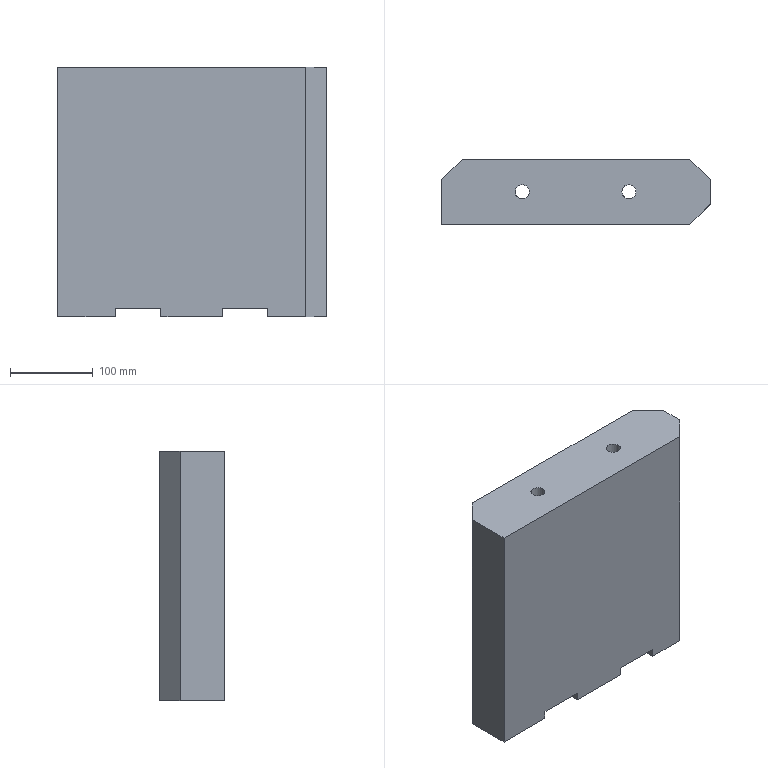Part | NX | features solid 2 | 1 solid | 23 faces | box 325 x 79 x 302 mm | volume 7112988 mm3 | plane 19 | cylinder 4 | commonest cylinder face diameters 17 x2 25 x2
STEP:
#1=CARTESIAN_POINT('',(-50.,-343.,178.));
#2=VERTEX_POINT('',#1);
#3=CARTESIAN_POINT('',(24.,-343.,178.));
#4=VERTEX_POINT('',#3);
#5=CARTESIAN_POINT('',(-177.942,-343.,178.));
#6=DIRECTION('',(1.,0.,0.));
#7=VECTOR('',#6,1000.);
#8=LINE('',#5,#7);
#9=EDGE_CURVE('',#2,#4,#8,.T.);
#10=ORIENTED_EDGE('',*,*,#9,.T.);
#11=CARTESIAN_POINT('',(24.,-422.,178.));
#12=VERTEX_POINT('',#11);
#13=CARTESIAN_POINT('',(24.,-420.217,178.));
#14=DIRECTION('',(0.,-1.,0.));
#15=VECTOR('',#14,1000.);
#16=LINE('',#13,#15);
#17=EDGE_CURVE('',#4,#12,#16,.T.);
#18=ORIENTED_EDGE('',*,*,#17,.T.);
#19=CARTESIAN_POINT('',(-50.,-422.,178.));
#20=VERTEX_POINT('',#19);
#21=CARTESIAN_POINT('',(-117.942,-422.,178.));
#22=DIRECTION('',(-1.,0.,0.));
#23=VECTOR('',#22,1000.);
#24=LINE('',#21,#23);
#25=EDGE_CURVE('',#12,#20,#24,.T.);
#26=ORIENTED_EDGE('',*,*,#25,.T.);
#27=CARTESIAN_POINT('',(-50.,-420.217,178.));
#28=DIRECTION('',(0.,-1.,0.));
#29=VECTOR('',#28,1000.);
#30=LINE('',#27,#29);
#31=EDGE_CURVE('',#2,#20,#30,.T.);
#32=ORIENTED_EDGE('',*,*,#31,.F.);
#33=EDGE_LOOP('',(#10,#18,#26,#32));
#34=FACE_BOUND('',#33,.T.);
#35=CARTESIAN_POINT('',(-177.942,-420.217,178.));
#36=DIRECTION('',(0.,0.,-1.));
#37=DIRECTION('',(0.,1.,0.));
#38=AXIS2_PLACEMENT_3D('',#35,#36,#37);
#39=PLANE('',#38);
#40=ADVANCED_FACE('',(#34),#39,.T.);
#41=CARTESIAN_POINT('',(-150.,-343.,178.));
#42=VERTEX_POINT('',#41);
#43=CARTESIAN_POINT('',(-105.,-343.,178.));
#44=VERTEX_POINT('',#43);
#45=CARTESIAN_POINT('',(-177.942,-343.,178.));
#46=DIRECTION('',(1.,0.,0.));
#47=VECTOR('',#46,1000.);
#48=LINE('',#45,#47);
#49=EDGE_CURVE('',#42,#44,#48,.T.);
#50=ORIENTED_EDGE('',*,*,#49,.T.);
#51=CARTESIAN_POINT('',(-105.,-422.,178.));
#52=VERTEX_POINT('',#51);
#53=CARTESIAN_POINT('',(-105.,-420.217,178.));
#54=DIRECTION('',(0.,-1.,0.));
#55=VECTOR('',#54,1000.);
#56=LINE('',#53,#55);
#57=EDGE_CURVE('',#44,#52,#56,.T.);
#58=ORIENTED_EDGE('',*,*,#57,.T.);
#59=CARTESIAN_POINT('',(-175.,-422.,178.));
#60=VERTEX_POINT('',#59);
#61=CARTESIAN_POINT('',(-117.942,-422.,178.));
#62=DIRECTION('',(-1.,0.,0.));
#63=VECTOR('',#62,1000.);
#64=LINE('',#61,#63);
#65=EDGE_CURVE('',#52,#60,#64,.T.);
#66=ORIENTED_EDGE('',*,*,#65,.T.);
#67=CARTESIAN_POINT('',(-175.,-368.,178.));
#68=VERTEX_POINT('',#67);
#69=CARTESIAN_POINT('',(-175.,-420.217,178.));
#70=DIRECTION('',(0.,1.,0.));
#71=VECTOR('',#70,1000.);
#72=LINE('',#69,#71);
#73=EDGE_CURVE('',#60,#68,#72,.T.);
#74=ORIENTED_EDGE('',*,*,#73,.T.);
#75=CARTESIAN_POINT('',(-202.579,-395.579,178.));
#76=DIRECTION('',(-0.7071,-0.7071,0.));
#77=VECTOR('',#76,1000.);
#78=LINE('',#75,#77);
#79=EDGE_CURVE('',#68,#42,#78,.F.);
#80=ORIENTED_EDGE('',*,*,#79,.T.);
#81=EDGE_LOOP('',(#50,#58,#66,#74,#80));
#82=FACE_BOUND('',#81,.T.);
#83=CARTESIAN_POINT('',(-177.942,-420.217,178.));
#84=DIRECTION('',(0.,0.,-1.));
#85=DIRECTION('',(0.,1.,0.));
#86=AXIS2_PLACEMENT_3D('',#83,#84,#85);
#87=PLANE('',#86);
#88=ADVANCED_FACE('',(#82),#87,.T.);
#89=CARTESIAN_POINT('',(24.,-422.,188.));
#90=VERTEX_POINT('',#89);
#91=CARTESIAN_POINT('',(79.,-422.,188.));
#92=VERTEX_POINT('',#91);
#93=CARTESIAN_POINT('',(24.489,-422.,188.));
#94=DIRECTION('',(-1.,0.,0.));
#95=VECTOR('',#94,1000.);
#96=LINE('',#93,#95);
#97=EDGE_CURVE('',#90,#92,#96,.F.);
#98=ORIENTED_EDGE('',*,*,#97,.T.);
#99=CARTESIAN_POINT('',(79.,-422.,178.));
#100=VERTEX_POINT('',#99);
#101=CARTESIAN_POINT('',(79.,-422.,192.6));
#102=DIRECTION('',(0.,0.,-1.));
#103=VECTOR('',#102,1000.);
#104=LINE('',#101,#103);
#105=EDGE_CURVE('',#92,#100,#104,.T.);
#106=ORIENTED_EDGE('',*,*,#105,.T.);
#107=CARTESIAN_POINT('',(125.,-422.,178.));
#108=VERTEX_POINT('',#107);
#109=CARTESIAN_POINT('',(-117.942,-422.,178.));
#110=DIRECTION('',(-1.,0.,0.));
#111=VECTOR('',#110,1000.);
#112=LINE('',#109,#111);
#113=EDGE_CURVE('',#108,#100,#112,.T.);
#114=ORIENTED_EDGE('',*,*,#113,.F.);
#115=CARTESIAN_POINT('',(125.,-422.,480.));
#116=VERTEX_POINT('',#115);
#117=CARTESIAN_POINT('',(125.,-422.,480.));
#118=DIRECTION('',(0.,0.,1.));
#119=VECTOR('',#118,1000.);
#120=LINE('',#117,#119);
#121=EDGE_CURVE('',#108,#116,#120,.T.);
#122=ORIENTED_EDGE('',*,*,#121,.T.);
#123=CARTESIAN_POINT('',(-175.,-422.,480.));
#124=VERTEX_POINT('',#123);
#125=CARTESIAN_POINT('',(-117.942,-422.,480.));
#126=DIRECTION('',(1.,0.,0.));
#127=VECTOR('',#126,1000.);
#128=LINE('',#125,#127);
#129=EDGE_CURVE('',#116,#124,#128,.F.);
#130=ORIENTED_EDGE('',*,*,#129,.T.);
#131=CARTESIAN_POINT('',(-175.,-422.,192.6));
#132=DIRECTION('',(0.,0.,1.));
#133=VECTOR('',#132,1000.);
#134=LINE('',#131,#133);
#135=EDGE_CURVE('',#60,#124,#134,.T.);
#136=ORIENTED_EDGE('',*,*,#135,.F.);
#137=ORIENTED_EDGE('',*,*,#65,.F.);
#138=CARTESIAN_POINT('',(-105.,-422.,188.));
#139=VERTEX_POINT('',#138);
#140=CARTESIAN_POINT('',(-105.,-422.,192.6));
#141=DIRECTION('',(0.,0.,-1.));
#142=VECTOR('',#141,1000.);
#143=LINE('',#140,#142);
#144=EDGE_CURVE('',#139,#52,#143,.T.);
#145=ORIENTED_EDGE('',*,*,#144,.F.);
#146=CARTESIAN_POINT('',(-50.,-422.,188.));
#147=VERTEX_POINT('',#146);
#148=CARTESIAN_POINT('',(-105.511,-422.,188.));
#149=DIRECTION('',(-1.,0.,0.));
#150=VECTOR('',#149,1000.);
#151=LINE('',#148,#150);
#152=EDGE_CURVE('',#139,#147,#151,.F.);
#153=ORIENTED_EDGE('',*,*,#152,.T.);
#154=CARTESIAN_POINT('',(-50.,-422.,192.6));
#155=DIRECTION('',(0.,0.,-1.));
#156=VECTOR('',#155,1000.);
#157=LINE('',#154,#156);
#158=EDGE_CURVE('',#147,#20,#157,.T.);
#159=ORIENTED_EDGE('',*,*,#158,.T.);
#160=ORIENTED_EDGE('',*,*,#25,.F.);
#161=CARTESIAN_POINT('',(24.,-422.,192.6));
#162=DIRECTION('',(0.,0.,-1.));
#163=VECTOR('',#162,1000.);
#164=LINE('',#161,#163);
#165=EDGE_CURVE('',#90,#12,#164,.T.);
#166=ORIENTED_EDGE('',*,*,#165,.F.);
#167=EDGE_LOOP('',(#98,#106,#114,#122,#130,#136,#137,#145,#153,#159,#160,#166));
#168=FACE_BOUND('',#167,.T.);
#169=CARTESIAN_POINT('',(-117.942,-422.,192.6));
#170=DIRECTION('',(0.,1.,0.));
#171=DIRECTION('',(0.,0.,1.));
#172=AXIS2_PLACEMENT_3D('',#169,#170,#171);
#173=PLANE('',#172);
#174=ADVANCED_FACE('',(#168),#173,.F.);
#175=CARTESIAN_POINT('',(-175.,-368.,480.));
#176=VERTEX_POINT('',#175);
#177=CARTESIAN_POINT('',(-175.,-420.217,480.));
#178=DIRECTION('',(0.,-1.,0.));
#179=VECTOR('',#178,1000.);
#180=LINE('',#177,#179);
#181=EDGE_CURVE('',#124,#176,#180,.F.);
#182=ORIENTED_EDGE('',*,*,#181,.T.);
#183=CARTESIAN_POINT('',(-175.,-368.,192.6));
#184=DIRECTION('',(0.,0.,-1.));
#185=VECTOR('',#184,1000.);
#186=LINE('',#183,#185);
#187=EDGE_CURVE('',#176,#68,#186,.T.);
#188=ORIENTED_EDGE('',*,*,#187,.T.);
#189=ORIENTED_EDGE('',*,*,#73,.F.);
#190=ORIENTED_EDGE('',*,*,#135,.T.);
#191=EDGE_LOOP('',(#182,#188,#189,#190));
#192=FACE_BOUND('',#191,.T.);
#193=CARTESIAN_POINT('',(-175.,-420.217,192.6));
#194=DIRECTION('',(1.,0.,0.));
#195=DIRECTION('',(0.,0.,-1.));
#196=AXIS2_PLACEMENT_3D('',#193,#194,#195);
#197=PLANE('',#196);
#198=ADVANCED_FACE('',(#192),#197,.F.);
#199=CARTESIAN_POINT('',(79.,-343.,178.));
#200=VERTEX_POINT('',#199);
#201=CARTESIAN_POINT('',(125.,-343.,178.));
#202=VERTEX_POINT('',#201);
#203=CARTESIAN_POINT('',(-177.942,-343.,178.));
#204=DIRECTION('',(1.,0.,0.));
#205=VECTOR('',#204,1000.);
#206=LINE('',#203,#205);
#207=EDGE_CURVE('',#200,#202,#206,.T.);
#208=ORIENTED_EDGE('',*,*,#207,.F.);
#209=CARTESIAN_POINT('',(79.,-343.,188.));
#210=VERTEX_POINT('',#209);
#211=CARTESIAN_POINT('',(79.,-343.,193.));
#212=DIRECTION('',(0.,0.,-1.));
#213=VECTOR('',#212,1000.);
#214=LINE('',#211,#213);
#215=EDGE_CURVE('',#210,#200,#214,.T.);
#216=ORIENTED_EDGE('',*,*,#215,.F.);
#217=CARTESIAN_POINT('',(24.,-343.,188.));
#218=VERTEX_POINT('',#217);
#219=CARTESIAN_POINT('',(-177.942,-343.,188.));
#220=DIRECTION('',(-1.,0.,0.));
#221=VECTOR('',#220,1000.);
#222=LINE('',#219,#221);
#223=EDGE_CURVE('',#218,#210,#222,.F.);
#224=ORIENTED_EDGE('',*,*,#223,.F.);
#225=CARTESIAN_POINT('',(24.,-343.,193.));
#226=DIRECTION('',(0.,0.,-1.));
#227=VECTOR('',#226,1000.);
#228=LINE('',#225,#227);
#229=EDGE_CURVE('',#218,#4,#228,.T.);
#230=ORIENTED_EDGE('',*,*,#229,.T.);
#231=ORIENTED_EDGE('',*,*,#9,.F.);
#232=CARTESIAN_POINT('',(-50.,-343.,188.));
#233=VERTEX_POINT('',#232);
#234=CARTESIAN_POINT('',(-50.,-343.,193.));
#235=DIRECTION('',(0.,0.,-1.));
#236=VECTOR('',#235,1000.);
#237=LINE('',#234,#236);
#238=EDGE_CURVE('',#233,#2,#237,.T.);
#239=ORIENTED_EDGE('',*,*,#238,.F.);
#240=CARTESIAN_POINT('',(-105.,-343.,188.));
#241=VERTEX_POINT('',#240);
#242=CARTESIAN_POINT('',(-177.942,-343.,188.));
#243=DIRECTION('',(-1.,0.,0.));
#244=VECTOR('',#243,1000.);
#245=LINE('',#242,#244);
#246=EDGE_CURVE('',#241,#233,#245,.F.);
#247=ORIENTED_EDGE('',*,*,#246,.F.);
#248=CARTESIAN_POINT('',(-105.,-343.,193.));
#249=DIRECTION('',(0.,0.,-1.));
#250=VECTOR('',#249,1000.);
#251=LINE('',#248,#250);
#252=EDGE_CURVE('',#241,#44,#251,.T.);
#253=ORIENTED_EDGE('',*,*,#252,.T.);
#254=ORIENTED_EDGE('',*,*,#49,.F.);
#255=CARTESIAN_POINT('',(-150.,-343.,480.));
#256=VERTEX_POINT('',#255);
#257=CARTESIAN_POINT('',(-150.,-343.,192.6));
#258=DIRECTION('',(0.,0.,1.));
#259=VECTOR('',#258,1000.);
#260=LINE('',#257,#259);
#261=EDGE_CURVE('',#42,#256,#260,.T.);
#262=ORIENTED_EDGE('',*,*,#261,.T.);
#263=CARTESIAN_POINT('',(125.,-343.,480.));
#264=VERTEX_POINT('',#263);
#265=CARTESIAN_POINT('',(-177.942,-343.,480.));
#266=DIRECTION('',(-1.,0.,0.));
#267=VECTOR('',#266,1000.);
#268=LINE('',#265,#267);
#269=EDGE_CURVE('',#256,#264,#268,.F.);
#270=ORIENTED_EDGE('',*,*,#269,.T.);
#271=CARTESIAN_POINT('',(125.,-343.,178.));
#272=DIRECTION('',(0.,0.,-1.));
#273=VECTOR('',#272,1000.);
#274=LINE('',#271,#273);
#275=EDGE_CURVE('',#264,#202,#274,.T.);
#276=ORIENTED_EDGE('',*,*,#275,.T.);
#277=EDGE_LOOP('',(#208,#216,#224,#230,#231,#239,#247,#253,#254,#262,#270,#276));
#278=FACE_BOUND('',#277,.T.);
#279=CARTESIAN_POINT('',(-177.942,-343.,192.6));
#280=DIRECTION('',(0.,-1.,0.));
#281=DIRECTION('',(0.,0.,-1.));
#282=AXIS2_PLACEMENT_3D('',#279,#280,#281);
#283=PLANE('',#282);
#284=ADVANCED_FACE('',(#278),#283,.F.);
#285=CARTESIAN_POINT('',(150.,-397.,178.));
#286=VERTEX_POINT('',#285);
#287=CARTESIAN_POINT('',(150.,-368.,178.));
#288=VERTEX_POINT('',#287);
#289=CARTESIAN_POINT('',(150.,-420.217,178.));
#290=DIRECTION('',(0.,1.,0.));
#291=VECTOR('',#290,1000.);
#292=LINE('',#289,#291);
#293=EDGE_CURVE('',#286,#288,#292,.T.);
#294=ORIENTED_EDGE('',*,*,#293,.T.);
#295=CARTESIAN_POINT('',(150.,-368.,480.));
#296=VERTEX_POINT('',#295);
#297=CARTESIAN_POINT('',(150.,-368.,480.));
#298=DIRECTION('',(0.,0.,1.));
#299=VECTOR('',#298,1000.);
#300=LINE('',#297,#299);
#301=EDGE_CURVE('',#288,#296,#300,.T.);
#302=ORIENTED_EDGE('',*,*,#301,.T.);
#303=CARTESIAN_POINT('',(150.,-397.,480.));
#304=VERTEX_POINT('',#303);
#305=CARTESIAN_POINT('',(150.,-420.217,480.));
#306=DIRECTION('',(0.,-1.,0.));
#307=VECTOR('',#306,1000.);
#308=LINE('',#305,#307);
#309=EDGE_CURVE('',#304,#296,#308,.F.);
#310=ORIENTED_EDGE('',*,*,#309,.F.);
#311=CARTESIAN_POINT('',(150.,-397.,178.));
#312=DIRECTION('',(0.,0.,-1.));
#313=VECTOR('',#312,1000.);
#314=LINE('',#311,#313);
#315=EDGE_CURVE('',#304,#286,#314,.T.);
#316=ORIENTED_EDGE('',*,*,#315,.T.);
#317=EDGE_LOOP('',(#294,#302,#310,#316));
#318=FACE_BOUND('',#317,.T.);
#319=CARTESIAN_POINT('',(150.,-420.217,192.6));
#320=DIRECTION('',(1.,0.,0.));
#321=DIRECTION('',(0.,0.,-1.));
#322=AXIS2_PLACEMENT_3D('',#319,#320,#321);
#323=PLANE('',#322);
#324=ADVANCED_FACE('',(#318),#323,.T.);
#325=CARTESIAN_POINT('',(79.,-420.217,178.));
#326=DIRECTION('',(0.,-1.,0.));
#327=VECTOR('',#326,1000.);
#328=LINE('',#325,#327);
#329=EDGE_CURVE('',#200,#100,#328,.T.);
#330=ORIENTED_EDGE('',*,*,#329,.F.);
#331=ORIENTED_EDGE('',*,*,#207,.T.);
#332=CARTESIAN_POINT('',(12.138,-230.138,178.));
#333=DIRECTION('',(0.7071,-0.7071,0.));
#334=VECTOR('',#333,1000.);
#335=LINE('',#332,#334);
#336=EDGE_CURVE('',#202,#288,#335,.T.);
#337=ORIENTED_EDGE('',*,*,#336,.T.);
#338=ORIENTED_EDGE('',*,*,#293,.F.);
#339=CARTESIAN_POINT('',(-25.579,-572.579,178.));
#340=DIRECTION('',(-0.7071,-0.7071,0.));
#341=VECTOR('',#340,1000.);
#342=LINE('',#339,#341);
#343=EDGE_CURVE('',#286,#108,#342,.T.);
#344=ORIENTED_EDGE('',*,*,#343,.T.);
#345=ORIENTED_EDGE('',*,*,#113,.T.);
#346=EDGE_LOOP('',(#330,#331,#337,#338,#344,#345));
#347=FACE_BOUND('',#346,.T.);
#348=CARTESIAN_POINT('',(-177.942,-420.217,178.));
#349=DIRECTION('',(0.,0.,-1.));
#350=DIRECTION('',(0.,1.,0.));
#351=AXIS2_PLACEMENT_3D('',#348,#349,#350);
#352=PLANE('',#351);
#353=ADVANCED_FACE('',(#347),#352,.T.);
#354=CARTESIAN_POINT('',(60.,-382.5,480.));
#355=VERTEX_POINT('',#354);
#356=CARTESIAN_POINT('',(51.5,-382.5,480.));
#357=DIRECTION('',(0.,0.,1.));
#358=DIRECTION('',(1.,0.,0.));
#359=AXIS2_PLACEMENT_3D('',#356,#357,#358);
#360=CIRCLE('',#359,8.5);
#361=EDGE_CURVE('',#355,#355,#360,.F.);
#362=ORIENTED_EDGE('',*,*,#361,.T.);
#363=EDGE_LOOP('',(#362));
#364=FACE_BOUND('',#363,.T.);
#365=CARTESIAN_POINT('',(-69.,-382.5,480.));
#366=VERTEX_POINT('',#365);
#367=CARTESIAN_POINT('',(-77.5,-382.5,480.));
#368=DIRECTION('',(0.,0.,1.));
#369=DIRECTION('',(1.,0.,0.));
#370=AXIS2_PLACEMENT_3D('',#367,#368,#369);
#371=CIRCLE('',#370,8.5);
#372=EDGE_CURVE('',#366,#366,#371,.F.);
#373=ORIENTED_EDGE('',*,*,#372,.T.);
#374=EDGE_LOOP('',(#373));
#375=FACE_BOUND('',#374,.T.);
#376=ORIENTED_EDGE('',*,*,#269,.F.);
#377=CARTESIAN_POINT('',(-150.,-343.,480.));
#378=DIRECTION('',(-0.7071,-0.7071,0.));
#379=VECTOR('',#378,1000.);
#380=LINE('',#377,#379);
#381=EDGE_CURVE('',#256,#176,#380,.T.);
#382=ORIENTED_EDGE('',*,*,#381,.T.);
#383=ORIENTED_EDGE('',*,*,#181,.F.);
#384=ORIENTED_EDGE('',*,*,#129,.F.);
#385=CARTESIAN_POINT('',(125.,-422.,480.));
#386=DIRECTION('',(-0.7071,-0.7071,0.));
#387=VECTOR('',#386,1000.);
#388=LINE('',#385,#387);
#389=EDGE_CURVE('',#116,#304,#388,.F.);
#390=ORIENTED_EDGE('',*,*,#389,.T.);
#391=ORIENTED_EDGE('',*,*,#309,.T.);
#392=CARTESIAN_POINT('',(150.,-368.,480.));
#393=DIRECTION('',(0.7071,-0.7071,0.));
#394=VECTOR('',#393,1000.);
#395=LINE('',#392,#394);
#396=EDGE_CURVE('',#296,#264,#395,.F.);
#397=ORIENTED_EDGE('',*,*,#396,.T.);
#398=EDGE_LOOP('',(#376,#382,#383,#384,#390,#391,#397));
#399=FACE_BOUND('',#398,.T.);
#400=CARTESIAN_POINT('',(238.333,388.333,480.));
#401=DIRECTION('',(0.,0.,1.));
#402=DIRECTION('',(0.,-1.,0.));
#403=AXIS2_PLACEMENT_3D('',#400,#401,#402);
#404=PLANE('',#403);
#405=ADVANCED_FACE('',(#364,#375,#399),#404,.T.);
#406=ORIENTED_EDGE('',*,*,#343,.F.);
#407=ORIENTED_EDGE('',*,*,#315,.F.);
#408=ORIENTED_EDGE('',*,*,#389,.F.);
#409=ORIENTED_EDGE('',*,*,#121,.F.);
#410=EDGE_LOOP('',(#406,#407,#408,#409));
#411=FACE_BOUND('',#410,.T.);
#412=CARTESIAN_POINT('',(125.,-422.,192.6));
#413=DIRECTION('',(0.7071,-0.7071,0.));
#414=DIRECTION('',(0.7071,0.7071,0.));
#415=AXIS2_PLACEMENT_3D('',#412,#413,#414);
#416=PLANE('',#415);
#417=ADVANCED_FACE('',(#411),#416,.T.);
#418=ORIENTED_EDGE('',*,*,#336,.F.);
#419=ORIENTED_EDGE('',*,*,#275,.F.);
#420=ORIENTED_EDGE('',*,*,#396,.F.);
#421=ORIENTED_EDGE('',*,*,#301,.F.);
#422=EDGE_LOOP('',(#418,#419,#420,#421));
#423=FACE_BOUND('',#422,.T.);
#424=CARTESIAN_POINT('',(150.,-368.,192.6));
#425=DIRECTION('',(0.7071,0.7071,0.));
#426=DIRECTION('',(-0.7071,0.7071,0.));
#427=AXIS2_PLACEMENT_3D('',#424,#425,#426);
#428=PLANE('',#427);
#429=ADVANCED_FACE('',(#423),#428,.T.);
#430=ORIENTED_EDGE('',*,*,#79,.F.);
#431=ORIENTED_EDGE('',*,*,#187,.F.);
#432=ORIENTED_EDGE('',*,*,#381,.F.);
#433=ORIENTED_EDGE('',*,*,#261,.F.);
#434=EDGE_LOOP('',(#430,#431,#432,#433));
#435=FACE_BOUND('',#434,.T.);
#436=CARTESIAN_POINT('',(-150.,-343.,192.6));
#437=DIRECTION('',(0.7071,-0.7071,0.));
#438=DIRECTION('',(0.7071,0.7071,0.));
#439=AXIS2_PLACEMENT_3D('',#436,#437,#438);
#440=PLANE('',#439);
#441=ADVANCED_FACE('',(#435),#440,.F.);
#442=CARTESIAN_POINT('',(-77.5,-395.,188.));
#443=VERTEX_POINT('',#442);
#444=CARTESIAN_POINT('',(-77.5,-382.5,188.));
#445=DIRECTION('',(0.,0.,1.));
#446=DIRECTION('',(0.,-1.,0.));
#447=AXIS2_PLACEMENT_3D('',#444,#445,#446);
#448=CIRCLE('',#447,12.5);
#449=EDGE_CURVE('',#443,#443,#448,.F.);
#450=ORIENTED_EDGE('',*,*,#449,.F.);
#451=EDGE_LOOP('',(#450));
#452=FACE_BOUND('',#451,.T.);
#453=ORIENTED_EDGE('',*,*,#152,.F.);
#454=CARTESIAN_POINT('',(-105.,-343.,188.));
#455=DIRECTION('',(0.,1.,0.));
#456=VECTOR('',#455,1000.);
#457=LINE('',#454,#456);
#458=EDGE_CURVE('',#241,#139,#457,.F.);
#459=ORIENTED_EDGE('',*,*,#458,.F.);
#460=ORIENTED_EDGE('',*,*,#246,.T.);
#461=CARTESIAN_POINT('',(-50.,-343.,188.));
#462=DIRECTION('',(0.,1.,0.));
#463=VECTOR('',#462,1000.);
#464=LINE('',#461,#463);
#465=EDGE_CURVE('',#233,#147,#464,.F.);
#466=ORIENTED_EDGE('',*,*,#465,.T.);
#467=EDGE_LOOP('',(#453,#459,#460,#466));
#468=FACE_BOUND('',#467,.T.);
#469=CARTESIAN_POINT('',(-105.511,-343.,188.));
#470=DIRECTION('',(0.,0.,1.));
#471=DIRECTION('',(0.,-1.,0.));
#472=AXIS2_PLACEMENT_3D('',#469,#470,#471);
#473=PLANE('',#472);
#474=ADVANCED_FACE('',(#452,#468),#473,.F.);
#475=ORIENTED_EDGE('',*,*,#31,.T.);
#476=ORIENTED_EDGE('',*,*,#158,.F.);
#477=ORIENTED_EDGE('',*,*,#465,.F.);
#478=ORIENTED_EDGE('',*,*,#238,.T.);
#479=EDGE_LOOP('',(#475,#476,#477,#478));
#480=FACE_BOUND('',#479,.T.);
#481=CARTESIAN_POINT('',(-50.,-343.,193.));
#482=DIRECTION('',(1.,0.,0.));
#483=DIRECTION('',(0.,1.,0.));
#484=AXIS2_PLACEMENT_3D('',#481,#482,#483);
#485=PLANE('',#484);
#486=ADVANCED_FACE('',(#480),#485,.F.);
#487=ORIENTED_EDGE('',*,*,#252,.F.);
#488=ORIENTED_EDGE('',*,*,#458,.T.);
#489=ORIENTED_EDGE('',*,*,#144,.T.);
#490=ORIENTED_EDGE('',*,*,#57,.F.);
#491=EDGE_LOOP('',(#487,#488,#489,#490));
#492=FACE_BOUND('',#491,.T.);
#493=CARTESIAN_POINT('',(-105.,-343.,193.));
#494=DIRECTION('',(1.,0.,0.));
#495=DIRECTION('',(0.,1.,0.));
#496=AXIS2_PLACEMENT_3D('',#493,#494,#495);
#497=PLANE('',#496);
#498=ADVANCED_FACE('',(#492),#497,.T.);
#499=CARTESIAN_POINT('',(51.5,-395.,188.));
#500=VERTEX_POINT('',#499);
#501=CARTESIAN_POINT('',(51.5,-382.5,188.));
#502=DIRECTION('',(0.,0.,1.));
#503=DIRECTION('',(0.,-1.,0.));
#504=AXIS2_PLACEMENT_3D('',#501,#502,#503);
#505=CIRCLE('',#504,12.5);
#506=EDGE_CURVE('',#500,#500,#505,.F.);
#507=ORIENTED_EDGE('',*,*,#506,.F.);
#508=EDGE_LOOP('',(#507));
#509=FACE_BOUND('',#508,.T.);
#510=ORIENTED_EDGE('',*,*,#97,.F.);
#511=CARTESIAN_POINT('',(24.,-343.,188.));
#512=DIRECTION('',(0.,1.,0.));
#513=VECTOR('',#512,1000.);
#514=LINE('',#511,#513);
#515=EDGE_CURVE('',#218,#90,#514,.F.);
#516=ORIENTED_EDGE('',*,*,#515,.F.);
#517=ORIENTED_EDGE('',*,*,#223,.T.);
#518=CARTESIAN_POINT('',(79.,-343.,188.));
#519=DIRECTION('',(0.,1.,0.));
#520=VECTOR('',#519,1000.);
#521=LINE('',#518,#520);
#522=EDGE_CURVE('',#210,#92,#521,.F.);
#523=ORIENTED_EDGE('',*,*,#522,.T.);
#524=EDGE_LOOP('',(#510,#516,#517,#523));
#525=FACE_BOUND('',#524,.T.);
#526=CARTESIAN_POINT('',(24.489,-343.,188.));
#527=DIRECTION('',(0.,0.,1.));
#528=DIRECTION('',(0.,-1.,0.));
#529=AXIS2_PLACEMENT_3D('',#526,#527,#528);
#530=PLANE('',#529);
#531=ADVANCED_FACE('',(#509,#525),#530,.F.);
#532=ORIENTED_EDGE('',*,*,#329,.T.);
#533=ORIENTED_EDGE('',*,*,#105,.F.);
#534=ORIENTED_EDGE('',*,*,#522,.F.);
#535=ORIENTED_EDGE('',*,*,#215,.T.);
#536=EDGE_LOOP('',(#532,#533,#534,#535));
#537=FACE_BOUND('',#536,.T.);
#538=CARTESIAN_POINT('',(79.,-343.,193.));
#539=DIRECTION('',(1.,0.,0.));
#540=DIRECTION('',(0.,1.,0.));
#541=AXIS2_PLACEMENT_3D('',#538,#539,#540);
#542=PLANE('',#541);
#543=ADVANCED_FACE('',(#537),#542,.F.);
#544=ORIENTED_EDGE('',*,*,#229,.F.);
#545=ORIENTED_EDGE('',*,*,#515,.T.);
#546=ORIENTED_EDGE('',*,*,#165,.T.);
#547=ORIENTED_EDGE('',*,*,#17,.F.);
#548=EDGE_LOOP('',(#544,#545,#546,#547));
#549=FACE_BOUND('',#548,.T.);
#550=CARTESIAN_POINT('',(24.,-343.,193.));
#551=DIRECTION('',(1.,0.,0.));
#552=DIRECTION('',(0.,1.,0.));
#553=AXIS2_PLACEMENT_3D('',#550,#551,#552);
#554=PLANE('',#553);
#555=ADVANCED_FACE('',(#549),#554,.T.);
#556=CARTESIAN_POINT('',(-77.5,-391.,450.));
#557=VERTEX_POINT('',#556);
#558=CARTESIAN_POINT('',(-77.5,-382.5,450.));
#559=DIRECTION('',(0.,0.,1.));
#560=DIRECTION('',(0.,-1.,0.));
#561=AXIS2_PLACEMENT_3D('',#558,#559,#560);
#562=CIRCLE('',#561,8.5);
#563=EDGE_CURVE('',#557,#557,#562,.F.);
#564=ORIENTED_EDGE('',*,*,#563,.T.);
#565=EDGE_LOOP('',(#564));
#566=FACE_BOUND('',#565,.T.);
#567=ORIENTED_EDGE('',*,*,#372,.F.);
#568=EDGE_LOOP('',(#567));
#569=FACE_BOUND('',#568,.T.);
#570=CARTESIAN_POINT('',(-77.5,-382.5,510.));
#571=DIRECTION('',(0.,0.,-1.));
#572=DIRECTION('',(0.,1.,0.));
#573=AXIS2_PLACEMENT_3D('',#570,#571,#572);
#574=CYLINDRICAL_SURFACE('',#573,8.5);
#575=ADVANCED_FACE('',(#566,#569),#574,.F.);
#576=ORIENTED_EDGE('',*,*,#563,.F.);
#577=EDGE_LOOP('',(#576));
#578=FACE_BOUND('',#577,.T.);
#579=CARTESIAN_POINT('',(-77.5,-370.,450.));
#580=VERTEX_POINT('',#579);
#581=CARTESIAN_POINT('',(-77.5,-382.5,450.));
#582=DIRECTION('',(0.,0.,-1.));
#583=DIRECTION('',(0.,1.,0.));
#584=AXIS2_PLACEMENT_3D('',#581,#582,#583);
#585=CIRCLE('',#584,12.5);
#586=EDGE_CURVE('',#580,#580,#585,.T.);
#587=ORIENTED_EDGE('',*,*,#586,.T.);
#588=EDGE_LOOP('',(#587));
#589=FACE_BOUND('',#588,.T.);
#590=CARTESIAN_POINT('',(-77.5,-382.5,450.));
#591=DIRECTION('',(0.,0.,1.));
#592=DIRECTION('',(0.,-1.,0.));
#593=AXIS2_PLACEMENT_3D('',#590,#591,#592);
#594=PLANE('',#593);
#595=ADVANCED_FACE('',(#578,#589),#594,.F.);
#596=ORIENTED_EDGE('',*,*,#449,.T.);
#597=EDGE_LOOP('',(#596));
#598=FACE_BOUND('',#597,.T.);
#599=ORIENTED_EDGE('',*,*,#586,.F.);
#600=EDGE_LOOP('',(#599));
#601=FACE_BOUND('',#600,.T.);
#602=CARTESIAN_POINT('',(-77.5,-382.5,450.));
#603=DIRECTION('',(0.,0.,-1.));
#604=DIRECTION('',(0.,1.,0.));
#605=AXIS2_PLACEMENT_3D('',#602,#603,#604);
#606=CYLINDRICAL_SURFACE('',#605,12.5);
#607=ADVANCED_FACE('',(#598,#601),#606,.F.);
#608=CARTESIAN_POINT('',(51.5,-391.,450.));
#609=VERTEX_POINT('',#608);
#610=CARTESIAN_POINT('',(51.5,-382.5,450.));
#611=DIRECTION('',(0.,0.,1.));
#612=DIRECTION('',(0.,-1.,0.));
#613=AXIS2_PLACEMENT_3D('',#610,#611,#612);
#614=CIRCLE('',#613,8.5);
#615=EDGE_CURVE('',#609,#609,#614,.F.);
#616=ORIENTED_EDGE('',*,*,#615,.T.);
#617=EDGE_LOOP('',(#616));
#618=FACE_BOUND('',#617,.T.);
#619=ORIENTED_EDGE('',*,*,#361,.F.);
#620=EDGE_LOOP('',(#619));
#621=FACE_BOUND('',#620,.T.);
#622=CARTESIAN_POINT('',(51.5,-382.5,510.));
#623=DIRECTION('',(0.,0.,-1.));
#624=DIRECTION('',(0.,1.,0.));
#625=AXIS2_PLACEMENT_3D('',#622,#623,#624);
#626=CYLINDRICAL_SURFACE('',#625,8.5);
#627=ADVANCED_FACE('',(#618,#621),#626,.F.);
#628=ORIENTED_EDGE('',*,*,#615,.F.);
#629=EDGE_LOOP('',(#628));
#630=FACE_BOUND('',#629,.T.);
#631=CARTESIAN_POINT('',(51.5,-370.,450.));
#632=VERTEX_POINT('',#631);
#633=CARTESIAN_POINT('',(51.5,-382.5,450.));
#634=DIRECTION('',(0.,0.,-1.));
#635=DIRECTION('',(0.,1.,0.));
#636=AXIS2_PLACEMENT_3D('',#633,#634,#635);
#637=CIRCLE('',#636,12.5);
#638=EDGE_CURVE('',#632,#632,#637,.T.);
#639=ORIENTED_EDGE('',*,*,#638,.T.);
#640=EDGE_LOOP('',(#639));
#641=FACE_BOUND('',#640,.T.);
#642=CARTESIAN_POINT('',(51.5,-382.5,450.));
#643=DIRECTION('',(0.,0.,1.));
#644=DIRECTION('',(0.,-1.,0.));
#645=AXIS2_PLACEMENT_3D('',#642,#643,#644);
#646=PLANE('',#645);
#647=ADVANCED_FACE('',(#630,#641),#646,.F.);
#648=ORIENTED_EDGE('',*,*,#506,.T.);
#649=EDGE_LOOP('',(#648));
#650=FACE_BOUND('',#649,.T.);
#651=ORIENTED_EDGE('',*,*,#638,.F.);
#652=EDGE_LOOP('',(#651));
#653=FACE_BOUND('',#652,.T.);
#654=CARTESIAN_POINT('',(51.5,-382.5,450.));
#655=DIRECTION('',(0.,0.,-1.));
#656=DIRECTION('',(0.,1.,0.));
#657=AXIS2_PLACEMENT_3D('',#654,#655,#656);
#658=CYLINDRICAL_SURFACE('',#657,12.5);
#659=ADVANCED_FACE('',(#650,#653),#658,.F.);
#660=CLOSED_SHELL('',(#40,#88,#174,#198,#284,#324,#353,#405,#417,#429,#441,#474,#486,#498,#531,#543,#555,#575,#595,#607,#627,#647,#659));
#661=MANIFOLD_SOLID_BREP('',#660);
#662=(LENGTH_UNIT()NAMED_UNIT(*)SI_UNIT(.MILLI.,.METRE.));
#663=UNCERTAINTY_MEASURE_WITH_UNIT(LENGTH_MEASURE(0.00001),#662,'','');
#664=(NAMED_UNIT(*)PLANE_ANGLE_UNIT()SI_UNIT($,.RADIAN.));
#665=(NAMED_UNIT(*)SI_UNIT($,.STERADIAN.)SOLID_ANGLE_UNIT());
#666=(GEOMETRIC_REPRESENTATION_CONTEXT(3)GLOBAL_UNCERTAINTY_ASSIGNED_CONTEXT((#663))GLOBAL_UNIT_ASSIGNED_CONTEXT((#662,#664,#665))REPRESENTATION_CONTEXT('',''));
#667=ADVANCED_BREP_SHAPE_REPRESENTATION('',(#661),#666);